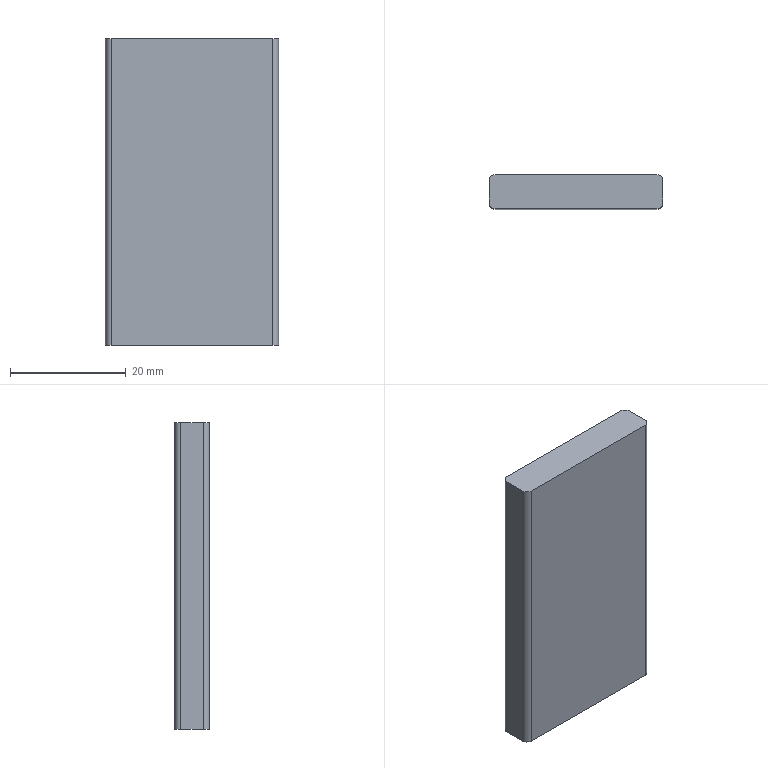Part | STEP file | 200 mesh_id30_xmt | 1 solid | 10 faces | box 29.97 x 5.97 x 53 mm | volume 9437 mm3 | plane 6 | cylinder 4 | commonest cylinder face diameters 2 x4
STEP:
#1=CARTESIAN_POINT('',(-17165.899,-4073.844,0.));
#2=VERTEX_POINT('',#1);
#3=CARTESIAN_POINT('',(-17193.869,-4073.844,0.));
#4=VERTEX_POINT('',#3);
#5=CARTESIAN_POINT('',(-17164.884,-4073.844,0.));
#6=DIRECTION('',(-1.,0.,0.));
#7=VECTOR('',#6,1.);
#8=LINE('',#5,#7);
#9=EDGE_CURVE('',#2,#4,#8,.T.);
#10=ORIENTED_EDGE('',*,*,#9,.T.);
#11=CARTESIAN_POINT('',(-17194.869,-4072.844,0.));
#12=VERTEX_POINT('',#11);
#13=CARTESIAN_POINT('',(-17193.869,-4072.844,0.));
#14=DIRECTION('',(0.,0.,-1.));
#15=DIRECTION('',(-1.,0.,0.));
#16=AXIS2_PLACEMENT_3D('',#13,#14,#15);
#17=CIRCLE('',#16,1.);
#18=EDGE_CURVE('',#4,#12,#17,.T.);
#19=ORIENTED_EDGE('',*,*,#18,.T.);
#20=CARTESIAN_POINT('',(-17194.869,-4068.874,0.));
#21=VERTEX_POINT('',#20);
#22=CARTESIAN_POINT('',(-17194.869,-4073.859,0.));
#23=DIRECTION('',(0.,1.,0.));
#24=VECTOR('',#23,1.);
#25=LINE('',#22,#24);
#26=EDGE_CURVE('',#12,#21,#25,.T.);
#27=ORIENTED_EDGE('',*,*,#26,.T.);
#28=CARTESIAN_POINT('',(-17193.869,-4067.874,0.));
#29=VERTEX_POINT('',#28);
#30=CARTESIAN_POINT('',(-17193.869,-4068.874,0.));
#31=DIRECTION('',(0.,0.,-1.));
#32=DIRECTION('',(-1.,0.,0.));
#33=AXIS2_PLACEMENT_3D('',#30,#31,#32);
#34=CIRCLE('',#33,1.);
#35=EDGE_CURVE('',#21,#29,#34,.T.);
#36=ORIENTED_EDGE('',*,*,#35,.T.);
#37=CARTESIAN_POINT('',(-17165.899,-4067.874,0.));
#38=VERTEX_POINT('',#37);
#39=CARTESIAN_POINT('',(-17194.884,-4067.874,0.));
#40=DIRECTION('',(1.,0.,0.));
#41=VECTOR('',#40,1.);
#42=LINE('',#39,#41);
#43=EDGE_CURVE('',#29,#38,#42,.T.);
#44=ORIENTED_EDGE('',*,*,#43,.T.);
#45=CARTESIAN_POINT('',(-17164.899,-4068.874,0.));
#46=VERTEX_POINT('',#45);
#47=CARTESIAN_POINT('',(-17165.899,-4068.874,0.));
#48=DIRECTION('',(0.,0.,-1.));
#49=DIRECTION('',(-1.,0.,0.));
#50=AXIS2_PLACEMENT_3D('',#47,#48,#49);
#51=CIRCLE('',#50,1.);
#52=EDGE_CURVE('',#38,#46,#51,.T.);
#53=ORIENTED_EDGE('',*,*,#52,.T.);
#54=CARTESIAN_POINT('',(-17164.899,-4072.844,0.));
#55=VERTEX_POINT('',#54);
#56=CARTESIAN_POINT('',(-17164.899,-4067.859,0.));
#57=DIRECTION('',(0.,-1.,0.));
#58=VECTOR('',#57,1.);
#59=LINE('',#56,#58);
#60=EDGE_CURVE('',#46,#55,#59,.T.);
#61=ORIENTED_EDGE('',*,*,#60,.T.);
#62=CARTESIAN_POINT('',(-17165.899,-4072.844,0.));
#63=DIRECTION('',(0.,0.,-1.));
#64=DIRECTION('',(-1.,0.,0.));
#65=AXIS2_PLACEMENT_3D('',#62,#63,#64);
#66=CIRCLE('',#65,1.);
#67=EDGE_CURVE('',#55,#2,#66,.T.);
#68=ORIENTED_EDGE('',*,*,#67,.T.);
#69=EDGE_LOOP('',(#10,#19,#27,#36,#44,#53,#61,#68));
#70=FACE_OUTER_BOUND('',#69,.T.);
#71=CARTESIAN_POINT('',(2237.268,-60.,0.));
#72=DIRECTION('',(0.,0.,-1.));
#73=DIRECTION('',(-1.,0.,0.));
#74=AXIS2_PLACEMENT_3D('',#71,#72,#73);
#75=PLANE('',#74);
#76=ADVANCED_FACE('',(#70),#75,.T.);
#77=CARTESIAN_POINT('',(-17165.899,-4073.844,53.));
#78=VERTEX_POINT('',#77);
#79=CARTESIAN_POINT('',(-17193.869,-4073.844,53.));
#80=VERTEX_POINT('',#79);
#81=CARTESIAN_POINT('',(-17164.884,-4073.844,53.));
#82=DIRECTION('',(-1.,0.,0.));
#83=VECTOR('',#82,1.);
#84=LINE('',#81,#83);
#85=EDGE_CURVE('',#78,#80,#84,.T.);
#86=ORIENTED_EDGE('',*,*,#85,.T.);
#87=CARTESIAN_POINT('',(-17193.869,-4073.844,-382.7));
#88=DIRECTION('',(0.,0.,-1.));
#89=VECTOR('',#88,1.);
#90=LINE('',#87,#89);
#91=EDGE_CURVE('',#80,#4,#90,.T.);
#92=ORIENTED_EDGE('',*,*,#91,.T.);
#93=ORIENTED_EDGE('',*,*,#9,.F.);
#94=CARTESIAN_POINT('',(-17165.899,-4073.844,-382.7));
#95=DIRECTION('',(0.,0.,1.));
#96=VECTOR('',#95,1.);
#97=LINE('',#94,#96);
#98=EDGE_CURVE('',#2,#78,#97,.T.);
#99=ORIENTED_EDGE('',*,*,#98,.T.);
#100=EDGE_LOOP('',(#86,#92,#93,#99));
#101=FACE_OUTER_BOUND('',#100,.T.);
#102=CARTESIAN_POINT('',(-17164.884,-4073.844,-382.7));
#103=DIRECTION('',(0.,1.,0.));
#104=DIRECTION('',(0.,0.,1.));
#105=AXIS2_PLACEMENT_3D('',#102,#103,#104);
#106=PLANE('',#105);
#107=ADVANCED_FACE('',(#101),#106,.F.);
#108=ORIENTED_EDGE('',*,*,#26,.F.);
#109=CARTESIAN_POINT('',(-17194.869,-4072.844,53.));
#110=VERTEX_POINT('',#109);
#111=CARTESIAN_POINT('',(-17194.869,-4072.844,-382.7));
#112=DIRECTION('',(0.,0.,1.));
#113=VECTOR('',#112,1.);
#114=LINE('',#111,#113);
#115=EDGE_CURVE('',#12,#110,#114,.T.);
#116=ORIENTED_EDGE('',*,*,#115,.T.);
#117=CARTESIAN_POINT('',(-17194.869,-4068.874,53.));
#118=VERTEX_POINT('',#117);
#119=CARTESIAN_POINT('',(-17194.869,-4073.859,53.));
#120=DIRECTION('',(0.,1.,0.));
#121=VECTOR('',#120,1.);
#122=LINE('',#119,#121);
#123=EDGE_CURVE('',#110,#118,#122,.T.);
#124=ORIENTED_EDGE('',*,*,#123,.T.);
#125=CARTESIAN_POINT('',(-17194.869,-4068.874,-382.7));
#126=DIRECTION('',(0.,0.,-1.));
#127=VECTOR('',#126,1.);
#128=LINE('',#125,#127);
#129=EDGE_CURVE('',#118,#21,#128,.T.);
#130=ORIENTED_EDGE('',*,*,#129,.T.);
#131=EDGE_LOOP('',(#108,#116,#124,#130));
#132=FACE_OUTER_BOUND('',#131,.T.);
#133=CARTESIAN_POINT('',(-17194.869,-4073.859,-382.7));
#134=DIRECTION('',(1.,0.,0.));
#135=DIRECTION('',(0.,0.,-1.));
#136=AXIS2_PLACEMENT_3D('',#133,#134,#135);
#137=PLANE('',#136);
#138=ADVANCED_FACE('',(#132),#137,.F.);
#139=ORIENTED_EDGE('',*,*,#43,.F.);
#140=CARTESIAN_POINT('',(-17193.869,-4067.874,53.));
#141=VERTEX_POINT('',#140);
#142=CARTESIAN_POINT('',(-17193.869,-4067.874,-382.7));
#143=DIRECTION('',(0.,0.,1.));
#144=VECTOR('',#143,1.);
#145=LINE('',#142,#144);
#146=EDGE_CURVE('',#29,#141,#145,.T.);
#147=ORIENTED_EDGE('',*,*,#146,.T.);
#148=CARTESIAN_POINT('',(-17165.899,-4067.874,53.));
#149=VERTEX_POINT('',#148);
#150=CARTESIAN_POINT('',(-17194.884,-4067.874,53.));
#151=DIRECTION('',(1.,0.,0.));
#152=VECTOR('',#151,1.);
#153=LINE('',#150,#152);
#154=EDGE_CURVE('',#141,#149,#153,.T.);
#155=ORIENTED_EDGE('',*,*,#154,.T.);
#156=CARTESIAN_POINT('',(-17165.899,-4067.874,-382.7));
#157=DIRECTION('',(0.,0.,-1.));
#158=VECTOR('',#157,1.);
#159=LINE('',#156,#158);
#160=EDGE_CURVE('',#149,#38,#159,.T.);
#161=ORIENTED_EDGE('',*,*,#160,.T.);
#162=EDGE_LOOP('',(#139,#147,#155,#161));
#163=FACE_OUTER_BOUND('',#162,.T.);
#164=CARTESIAN_POINT('',(-17194.884,-4067.874,-382.7));
#165=DIRECTION('',(0.,-1.,0.));
#166=DIRECTION('',(0.,0.,-1.));
#167=AXIS2_PLACEMENT_3D('',#164,#165,#166);
#168=PLANE('',#167);
#169=ADVANCED_FACE('',(#163),#168,.F.);
#170=CARTESIAN_POINT('',(-17164.899,-4068.874,53.));
#171=VERTEX_POINT('',#170);
#172=CARTESIAN_POINT('',(-17164.899,-4072.844,53.));
#173=VERTEX_POINT('',#172);
#174=CARTESIAN_POINT('',(-17164.899,-4067.859,53.));
#175=DIRECTION('',(0.,-1.,0.));
#176=VECTOR('',#175,1.);
#177=LINE('',#174,#176);
#178=EDGE_CURVE('',#171,#173,#177,.T.);
#179=ORIENTED_EDGE('',*,*,#178,.T.);
#180=CARTESIAN_POINT('',(-17164.899,-4072.844,-382.7));
#181=DIRECTION('',(0.,0.,-1.));
#182=VECTOR('',#181,1.);
#183=LINE('',#180,#182);
#184=EDGE_CURVE('',#173,#55,#183,.T.);
#185=ORIENTED_EDGE('',*,*,#184,.T.);
#186=ORIENTED_EDGE('',*,*,#60,.F.);
#187=CARTESIAN_POINT('',(-17164.899,-4068.874,-382.7));
#188=DIRECTION('',(0.,0.,1.));
#189=VECTOR('',#188,1.);
#190=LINE('',#187,#189);
#191=EDGE_CURVE('',#46,#171,#190,.T.);
#192=ORIENTED_EDGE('',*,*,#191,.T.);
#193=EDGE_LOOP('',(#179,#185,#186,#192));
#194=FACE_OUTER_BOUND('',#193,.T.);
#195=CARTESIAN_POINT('',(-17164.899,-4067.859,-382.7));
#196=DIRECTION('',(-1.,0.,0.));
#197=DIRECTION('',(0.,0.,1.));
#198=AXIS2_PLACEMENT_3D('',#195,#196,#197);
#199=PLANE('',#198);
#200=ADVANCED_FACE('',(#194),#199,.F.);
#201=ORIENTED_EDGE('',*,*,#123,.F.);
#202=CARTESIAN_POINT('',(-17193.869,-4072.844,53.));
#203=DIRECTION('',(0.,0.,1.));
#204=DIRECTION('',(-1.,0.,0.));
#205=AXIS2_PLACEMENT_3D('',#202,#203,#204);
#206=CIRCLE('',#205,1.);
#207=EDGE_CURVE('',#110,#80,#206,.T.);
#208=ORIENTED_EDGE('',*,*,#207,.T.);
#209=ORIENTED_EDGE('',*,*,#85,.F.);
#210=CARTESIAN_POINT('',(-17165.899,-4072.844,53.));
#211=DIRECTION('',(0.,0.,1.));
#212=DIRECTION('',(-1.,0.,0.));
#213=AXIS2_PLACEMENT_3D('',#210,#211,#212);
#214=CIRCLE('',#213,1.);
#215=EDGE_CURVE('',#78,#173,#214,.T.);
#216=ORIENTED_EDGE('',*,*,#215,.T.);
#217=ORIENTED_EDGE('',*,*,#178,.F.);
#218=CARTESIAN_POINT('',(-17165.899,-4068.874,53.));
#219=DIRECTION('',(0.,0.,1.));
#220=DIRECTION('',(-1.,0.,0.));
#221=AXIS2_PLACEMENT_3D('',#218,#219,#220);
#222=CIRCLE('',#221,1.);
#223=EDGE_CURVE('',#171,#149,#222,.T.);
#224=ORIENTED_EDGE('',*,*,#223,.T.);
#225=ORIENTED_EDGE('',*,*,#154,.F.);
#226=CARTESIAN_POINT('',(-17193.869,-4068.874,53.));
#227=DIRECTION('',(0.,0.,1.));
#228=DIRECTION('',(-1.,0.,0.));
#229=AXIS2_PLACEMENT_3D('',#226,#227,#228);
#230=CIRCLE('',#229,1.);
#231=EDGE_CURVE('',#141,#118,#230,.T.);
#232=ORIENTED_EDGE('',*,*,#231,.T.);
#233=EDGE_LOOP('',(#201,#208,#209,#216,#217,#224,#225,#232));
#234=FACE_OUTER_BOUND('',#233,.T.);
#235=CARTESIAN_POINT('',(0.,-60.,53.));
#236=DIRECTION('',(0.,0.,-1.));
#237=DIRECTION('',(-1.,0.,0.));
#238=AXIS2_PLACEMENT_3D('',#235,#236,#237);
#239=PLANE('',#238);
#240=ADVANCED_FACE('',(#234),#239,.F.);
#241=ORIENTED_EDGE('',*,*,#18,.F.);
#242=ORIENTED_EDGE('',*,*,#91,.F.);
#243=ORIENTED_EDGE('',*,*,#207,.F.);
#244=ORIENTED_EDGE('',*,*,#115,.F.);
#245=EDGE_LOOP('',(#241,#242,#243,#244));
#246=FACE_OUTER_BOUND('',#245,.T.);
#247=CARTESIAN_POINT('',(-17193.869,-4072.844,-382.7));
#248=DIRECTION('',(0.,0.,1.));
#249=DIRECTION('',(1.,0.,0.));
#250=AXIS2_PLACEMENT_3D('',#247,#248,#249);
#251=CYLINDRICAL_SURFACE('',#250,1.);
#252=ADVANCED_FACE('',(#246),#251,.T.);
#253=ORIENTED_EDGE('',*,*,#35,.F.);
#254=ORIENTED_EDGE('',*,*,#129,.F.);
#255=ORIENTED_EDGE('',*,*,#231,.F.);
#256=ORIENTED_EDGE('',*,*,#146,.F.);
#257=EDGE_LOOP('',(#253,#254,#255,#256));
#258=FACE_OUTER_BOUND('',#257,.T.);
#259=CARTESIAN_POINT('',(-17193.869,-4068.874,-382.7));
#260=DIRECTION('',(0.,0.,1.));
#261=DIRECTION('',(1.,0.,0.));
#262=AXIS2_PLACEMENT_3D('',#259,#260,#261);
#263=CYLINDRICAL_SURFACE('',#262,1.);
#264=ADVANCED_FACE('',(#258),#263,.T.);
#265=ORIENTED_EDGE('',*,*,#67,.F.);
#266=ORIENTED_EDGE('',*,*,#184,.F.);
#267=ORIENTED_EDGE('',*,*,#215,.F.);
#268=ORIENTED_EDGE('',*,*,#98,.F.);
#269=EDGE_LOOP('',(#265,#266,#267,#268));
#270=FACE_OUTER_BOUND('',#269,.T.);
#271=CARTESIAN_POINT('',(-17165.899,-4072.844,-382.7));
#272=DIRECTION('',(0.,0.,1.));
#273=DIRECTION('',(1.,0.,0.));
#274=AXIS2_PLACEMENT_3D('',#271,#272,#273);
#275=CYLINDRICAL_SURFACE('',#274,1.);
#276=ADVANCED_FACE('',(#270),#275,.T.);
#277=ORIENTED_EDGE('',*,*,#52,.F.);
#278=ORIENTED_EDGE('',*,*,#160,.F.);
#279=ORIENTED_EDGE('',*,*,#223,.F.);
#280=ORIENTED_EDGE('',*,*,#191,.F.);
#281=EDGE_LOOP('',(#277,#278,#279,#280));
#282=FACE_OUTER_BOUND('',#281,.T.);
#283=CARTESIAN_POINT('',(-17165.899,-4068.874,-382.7));
#284=DIRECTION('',(0.,0.,1.));
#285=DIRECTION('',(1.,0.,0.));
#286=AXIS2_PLACEMENT_3D('',#283,#284,#285);
#287=CYLINDRICAL_SURFACE('',#286,1.);
#288=ADVANCED_FACE('',(#282),#287,.T.);
#289=CLOSED_SHELL('',(#76,#107,#138,#169,#200,#240,#252,#264,#276,#288));
#290=MANIFOLD_SOLID_BREP('',#289);
#291=(LENGTH_UNIT()NAMED_UNIT(*)SI_UNIT(.MILLI.,.METRE.));
#292=UNCERTAINTY_MEASURE_WITH_UNIT(LENGTH_MEASURE(0.00002),#291,'','');
#293=(NAMED_UNIT(*)PLANE_ANGLE_UNIT()SI_UNIT($,.RADIAN.));
#294=PLANE_ANGLE_MEASURE_WITH_UNIT(PLANE_ANGLE_MEASURE(0.01745),#293);
#295=DIMENSIONAL_EXPONENTS(0.,0.,0.,0.,0.,0.,0.);
#296=(CONVERSION_BASED_UNIT('DEGREE',#294)NAMED_UNIT(#295)PLANE_ANGLE_UNIT());
#297=(NAMED_UNIT(*)SI_UNIT($,.STERADIAN.)SOLID_ANGLE_UNIT());
#298=(GEOMETRIC_REPRESENTATION_CONTEXT(3)GLOBAL_UNCERTAINTY_ASSIGNED_CONTEXT((#292))GLOBAL_UNIT_ASSIGNED_CONTEXT((#291,#296,#297))REPRESENTATION_CONTEXT('',''));
#299=ADVANCED_BREP_SHAPE_REPRESENTATION('',(#290),#298);